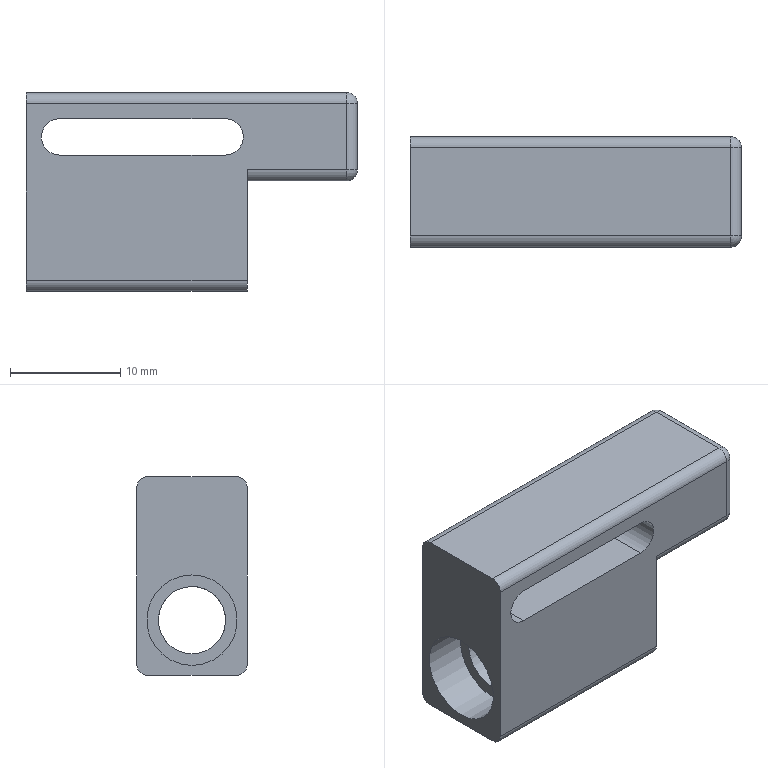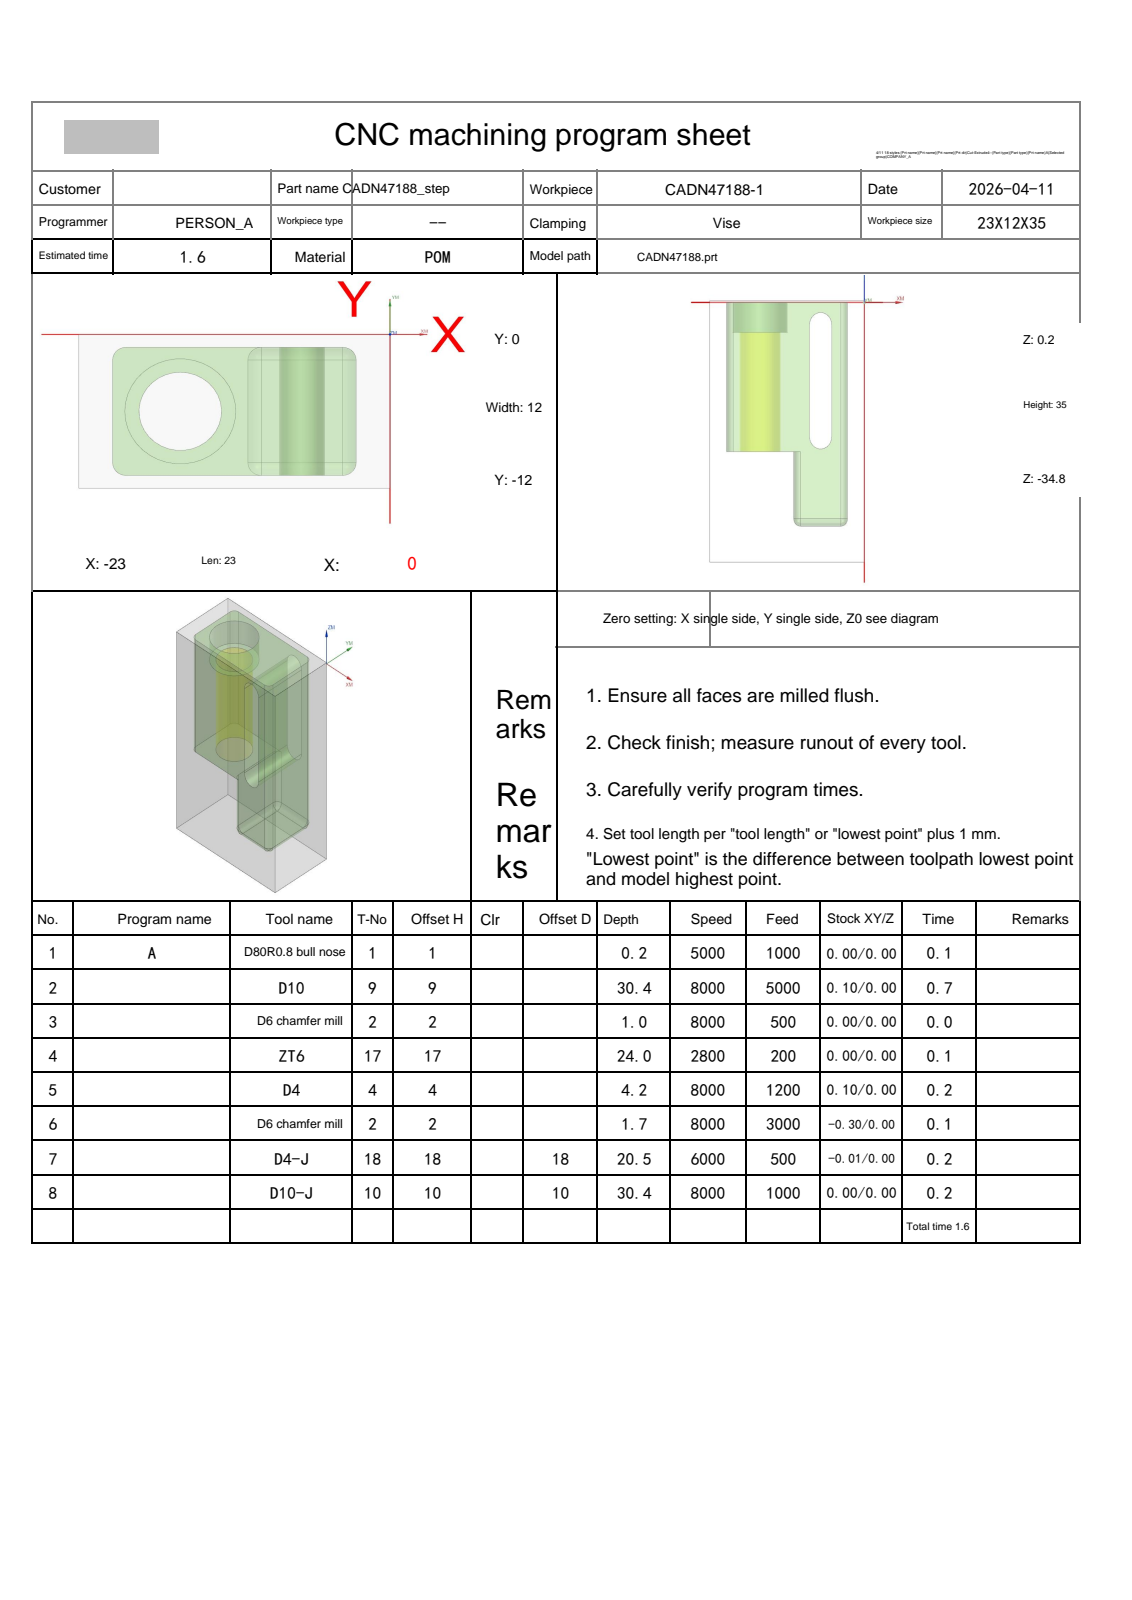NC program | NX | posted by the shop | part box 30 x 10 x 18 mm
Whole program:
%
O0001
(Machine time: 3.23 MIN)
(===Total Tool:7===)
(T1=D80R0.8 bull nose D=80.  R=0.8  D-  H01 Z=-0.   )
(T9=D10     D=10.  R=0.   D-  H09 Z=-30.2 )
(T2=D6 chamfer mill   D=6.   R=0.   D-  H02 Z=-1.5  )
(T17=ZT6    D=6.   DR_a=118 D-  H17 Z=-23.8 )
(T4=D4      D=4.   R=0.   D-  H04 Z=-4.   )
(T18=D4-J   D=4.   R=0.   D18 H18 Z=-20.3 )
(T10=D10-J  D=10.  R=0.   D10 H10 Z=-30.2 )
G80 G90 G17 G49 G40
G91 G28 Z0
M01
N1 T01 M06
(D80R0.8 bull nose  D=80. R=0.8 H=01 ce=0.00 di=0.00)
G00 G90 G54 X-65.5 Y-6. M03 S5000
G43 H01 Z20.
M08
Z2.
G01 Z0.0 F1000.
X-60.5
X37.5
X42.5
Z2.
G00 Z20.
G91 G28 Z0.0
M05
M09
G91 G28 Z0.0
M01
N2 T09 M06
(D10  D=10. R=0. H=09 ce=0.10 di=0.00)
G00 G90 G54 X-11.5 Y4.1 M03 S8000
G43 H09 Z20.
M08
Z.5
G01 X-3.5 Z.427 F5000.
G02 X2.6 Y-2. Z.34 I0.0 J-6.1
G01 Y-10. Z.267
G02 X-3.5 Y-16.1 Z.179 I-6.1 J0.0
G01 X-19.5 Z.033
G02 X-25.6 Y-10. Z-.054 I0.0 J6.1
G01 Y-2. Z-.127
G02 X-19.5 Y4.1 Z-.214 I6.1 J0.0
G01 X-3.5 Z-.36
G02 X2.6 Y-2. Z-.448 I0.0 J-6.1
G01 Y-10. Z-.52
G02 X-3.5 Y-16.1 Z-.608 I-6.1 J0.0
G01 X-19.5 Z-.754
G02 X-25.6 Y-10. Z-.841 I0.0 J6.1
G01 Y-2. Z-.914
G02 X-19.5 Y4.1 Z-1.001 I6.1 J0.0
G01 X-3.5 Z-1.147
G02 X2.6 Y-2. Z-1.235 I0.0 J-6.1
G01 Y-10. Z-1.308
G02 X-3.5 Y-16.1 Z-1.395 I-6.1 J0.0
G01 X-19.5 Z-1.541
G02 X-25.6 Y-10. Z-1.628 I0.0 J6.1
G01 Y-2. Z-1.701
G02 X-19.5 Y4.1 Z-1.789 I6.1 J0.0
G01 X-3.5 Z-1.934
G02 X2.6 Y-2. Z-2.022 I0.0 J-6.1
G01 Y-10. Z-2.095
G02 X-3.5 Y-16.1 Z-2.182 I-6.1 J0.0
G01 X-19.5 Z-2.328
G02 X-25.6 Y-10. Z-2.415 I0.0 J6.1
G01 Y-2. Z-2.488
G02 X-19.5 Y4.1 Z-2.576 I6.1 J0.0
G01 X-3.5 Z-2.722
G02 X2.6 Y-2. Z-2.809 I0.0 J-6.1
G01 Y-10. Z-2.882
G02 X-3.5 Y-16.1 Z-2.969 I-6.1 J0.0
G01 X-19.5 Z-3.115
G02 X-25.6 Y-10. Z-3.203 I0.0 J6.1
G01 Y-2. Z-3.276
G02 X-19.5 Y4.1 Z-3.363 I6.1 J0.0
G01 X-3.5 Z-3.509
G02 X2.6 Y-2. Z-3.596 I0.0 J-6.1
G01 Y-10. Z-3.669
G02 X-3.5 Y-16.1 Z-3.757 I-6.1 J0.0
G01 X-19.5 Z-3.902
G02 X-25.6 Y-10. Z-3.99 I0.0 J6.1
G01 Y-2. Z-4.063
G02 X-19.5 Y4.1 Z-4.15 I6.1 J0.0
G01 X-3.5 Z-4.296
G02 X2.6 Y-2. Z-4.383 I0.0 J-6.1
G01 Y-10. Z-4.456
G02 X-3.5 Y-16.1 Z-4.544 I-6.1 J0.0
G01 X-19.5 Z-4.69
G02 X-25.6 Y-10. Z-4.777 I0.0 J6.1
G01 Y-2. Z-4.85
G02 X-19.5 Y4.1 Z-4.937 I6.1 J0.0
G01 X-3.5 Z-5.083
G02 X2.6 Y-2. Z-5.171 I0.0 J-6.1
G01 Y-10. Z-5.244
G02 X-3.5 Y-16.1 Z-5.331 I-6.1 J0.0
G01 X-19.5 Z-5.477
G02 X-25.6 Y-10. Z-5.564 I0.0 J6.1
G01 Y-2. Z-5.637
G02 X-19.5 Y4.1 Z-5.724 I6.1 J0.0
G01 X-3.5 Z-5.87
G02 X2.6 Y-2. Z-5.958 I0.0 J-6.1
G01 Y-10. Z-6.031
G02 X-3.5 Y-16.1 Z-6.118 I-6.1 J0.0
G01 X-19.5 Z-6.264
G02 X-25.6 Y-10. Z-6.351 I0.0 J6.1
G01 Y-2. Z-6.424
G02 X-19.5 Y4.1 Z-6.512 I6.1 J0.0
G01 X-3.5 Z-6.658
G02 X2.6 Y-2. Z-6.745 I0.0 J-6.1
G01 Y-10. Z-6.818
G02 X-3.5 Y-16.1 Z-6.905 I-6.1 J0.0
G01 X-19.5 Z-7.051
G02 X-25.6 Y-10. Z-7.139 I0.0 J6.1
G01 Y-2. Z-7.211
G02 X-19.5 Y4.1 Z-7.299 I6.1 J0.0
G01 X-3.5 Z-7.445
G02 X2.6 Y-2. Z-7.532 I0.0 J-6.1
G01 Y-10. Z-7.605
G02 X-3.5 Y-16.1 Z-7.692 I-6.1 J0.0
G01 X-19.5 Z-7.838
G02 X-25.6 Y-10. Z-7.926 I0.0 J6.1
G01 Y-2. Z-7.999
G02 X-19.5 Y4.1 Z-8.086 I6.1 J0.0
G01 X-3.5 Z-8.232
G02 X2.6 Y-2. Z-8.319 I0.0 J-6.1
G01 Y-10. Z-8.392
G02 X-3.5 Y-16.1 Z-8.48 I-6.1 J0.0
G01 X-19.5 Z-8.626
G02 X-25.6 Y-10. Z-8.713 I0.0 J6.1
G01 Y-2. Z-8.786
G02 X-19.5 Y4.1 Z-8.873 I6.1 J0.0
G01 X-3.5 Z-9.019
G02 X2.6 Y-2. Z-9.106 I0.0 J-6.1
G01 Y-10. Z-9.179
G02 X-3.5 Y-16.1 Z-9.267 I-6.1 J0.0
G01 X-19.5 Z-9.413
G02 X-25.6 Y-10. Z-9.5 I0.0 J6.1
G01 Y-2. Z-9.573
G02 X-19.5 Y4.1 Z-9.66 I6.1 J0.0
G01 X-3.5 Z-9.806
G02 X2.6 Y-2. Z-9.894 I0.0 J-6.1
G01 Y-10. Z-9.967
G02 X-3.5 Y-16.1 Z-10.054 I-6.1 J0.0
G01 X-19.5 Z-10.2
G02 X-25.6 Y-10. Z-10.287 I0.0 J6.1
G01 Y-2. Z-10.36
G02 X-19.5 Y4.1 Z-10.448 I6.1 J0.0
G01 X-3.5 Z-10.593
G02 X2.6 Y-2. Z-10.681 I0.0 J-6.1
G01 Y-10. Z-10.754
G02 X-3.5 Y-16.1 Z-10.841 I-6.1 J0.0
G01 X-19.5 Z-10.987
G02 X-25.6 Y-10. Z-11.074 I0.0 J6.1
G01 Y-2. Z-11.147
G02 X-19.5 Y4.1 Z-11.235 I6.1 J0.0
G01 X-3.5 Z-11.381
G02 X2.6 Y-2. Z-11.468 I0.0 J-6.1
G01 Y-10. Z-11.541
G02 X-3.5 Y-16.1 Z-11.628 I-6.1 J0.0
G01 X-19.5 Z-11.774
G02 X-25.6 Y-10. Z-11.862 I0.0 J6.1
G01 Y-2. Z-11.935
G02 X-19.5 Y4.1 Z-12.022 I6.1 J0.0
G01 X-3.5 Z-12.168
G02 X2.6 Y-2. Z-12.255 I0.0 J-6.1
G01 Y-10. Z-12.328
G02 X-3.5 Y-16.1 Z-12.416 I-6.1 J0.0
G01 X-19.5 Z-12.561
G02 X-25.6 Y-10. Z-12.649 I0.0 J6.1
G01 Y-2. Z-12.722
G02 X-19.5 Y4.1 Z-12.809 I6.1 J0.0
G01 X-3.5 Z-12.955
G02 X2.6 Y-2. Z-13.042 I0.0 J-6.1
G01 Y-10. Z-13.115
G02 X-3.5 Y-16.1 Z-13.203 I-6.1 J0.0
G01 X-19.5 Z-13.349
G02 X-25.6 Y-10. Z-13.436 I0.0 J6.1
G01 Y-2. Z-13.509
G02 X-19.5 Y4.1 Z-13.596 I6.1 J0.0
G01 X-3.5 Z-13.742
G02 X2.6 Y-2. Z-13.83 I0.0 J-6.1
G01 Y-10. Z-13.903
G02 X-3.5 Y-16.1 Z-13.99 I-6.1 J0.0
G01 X-19.5 Z-14.136
G02 X-25.6 Y-10. Z-14.223 I0.0 J6.1
G01 Y-2. Z-14.296
G02 X-19.5 Y4.1 Z-14.383 I6.1 J0.0
G01 X-3.5 Z-14.529
G02 X2.6 Y-2. Z-14.617 I0.0 J-6.1
G01 Y-10. Z-14.69
G02 X-3.5 Y-16.1 Z-14.777 I-6.1 J0.0
G01 X-19.5 Z-14.923
G02 X-25.6 Y-10. Z-15.01 I0.0 J6.1
G01 Y-2. Z-15.083
G02 X-19.5 Y4.1 Z-15.171 I6.1 J0.0
G01 X-3.5 Z-15.317
G02 X2.6 Y-2. Z-15.404 I0.0 J-6.1
G01 Y-10. Z-15.477
G02 X-3.5 Y-16.1 Z-15.564 I-6.1 J0.0
G01 X-19.5 Z-15.71
G02 X-25.6 Y-10. Z-15.798 I0.0 J6.1
G01 Y-2. Z-15.87
G02 X-19.5 Y4.1 Z-15.958 I6.1 J0.0
G01 X-3.5 Z-16.104
G02 X2.6 Y-2. Z-16.191 I0.0 J-6.1
G01 Y-10. Z-16.264
G02 X-3.5 Y-16.1 Z-16.351 I-6.1 J0.0
G01 X-19.5 Z-16.497
G02 X-25.6 Y-10. Z-16.585 I0.0 J6.1
G01 Y-2. Z-16.658
G02 X-19.5 Y4.1 Z-16.745 I6.1 J0.0
G01 X-3.5 Z-16.891
G02 X2.6 Y-2. Z-16.978 I0.0 J-6.1
G01 Y-10. Z-17.051
G02 X-3.5 Y-16.1 Z-17.139 I-6.1 J0.0
G01 X-19.5 Z-17.284
G02 X-25.6 Y-10. Z-17.372 I0.0 J6.1
G01 Y-2. Z-17.445
G02 X-19.5 Y4.1 Z-17.532 I6.1 J0.0
G01 X-3.5 Z-17.678
G02 X2.6 Y-2. Z-17.765 I0.0 J-6.1
G01 Y-10. Z-17.838
G02 X-3.5 Y-16.1 Z-17.926 I-6.1 J0.0
G01 X-19.5 Z-18.072
G02 X-25.6 Y-10. Z-18.159 I0.0 J6.1
G01 Y-2. Z-18.232
G02 X-19.5 Y4.1 Z-18.319 I6.1 J0.0
G01 X-3.5 Z-18.465
G02 X2.6 Y-2. Z-18.553 I0.0 J-6.1
G01 Y-10. Z-18.626
G02 X-3.5 Y-16.1 Z-18.713 I-6.1 J0.0
G01 X-19.5 Z-18.859
G02 X-25.6 Y-10. Z-18.946 I0.0 J6.1
G01 Y-2. Z-19.019
G02 X-19.5 Y4.1 Z-19.107 I6.1 J0.0
G01 X-3.5 Z-19.252
G02 X2.6 Y-2. Z-19.34 I0.0 J-6.1
G01 Y-10. Z-19.413
G02 X-3.5 Y-16.1 Z-19.5 I-6.1 J0.0
G01 X-19.5 Z-19.646
G02 X-25.6 Y-10. Z-19.733 I0.0 J6.1
G01 Y-2. Z-19.806
G02 X-19.5 Y4.1 Z-19.894 I6.1 J0.0
G01 X-3.5 Z-20.04
G02 X2.6 Y-2. Z-20.127 I0.0 J-6.1
G01 Y-10. Z-20.2
G02 X-3.5 Y-16.1 Z-20.287 I-6.1 J0.0
G01 X-19.5 Z-20.433
G02 X-25.6 Y-10. Z-20.521 I0.0 J6.1
G01 Y-2. Z-20.594
G02 X-19.5 Y4.1 Z-20.681 I6.1 J0.0
G01 X-3.5 Z-20.827
G02 X2.6 Y-2. Z-20.914 I0.0 J-6.1
G01 Y-10. Z-20.987
G02 X-3.5 Y-16.1 Z-21.074 I-6.1 J0.0
G01 X-19.5 Z-21.22
G02 X-25.6 Y-10. Z-21.308 I0.0 J6.1
G01 Y-2. Z-21.381
G02 X-19.5 Y4.1 Z-21.468 I6.1 J0.0
G01 X-3.5 Z-21.614
G02 X2.6 Y-2. Z-21.701 I0.0 J-6.1
G01 Y-10. Z-21.774
G02 X-3.5 Y-16.1 Z-21.862 I-6.1 J0.0
G01 X-19.5 Z-22.008
G02 X-25.6 Y-10. Z-22.095 I0.0 J6.1
G01 Y-2. Z-22.168
G02 X-19.5 Y4.1 Z-22.255 I6.1 J0.0
G01 X-3.5 Z-22.401
G02 X2.6 Y-2. Z-22.489 I0.0 J-6.1
G01 Y-10. Z-22.561
G02 X-3.5 Y-16.1 Z-22.649 I-6.1 J0.0
G01 X-19.5 Z-22.795
G02 X-25.6 Y-10. Z-22.882 I0.0 J6.1
G01 Y-2. Z-22.955
G02 X-19.5 Y4.1 Z-23.042 I6.1 J0.0
G01 X-3.5 Z-23.188
G02 X2.6 Y-2. Z-23.276 I0.0 J-6.1
G01 Y-10. Z-23.349
G02 X-3.5 Y-16.1 Z-23.436 I-6.1 J0.0
G01 X-19.5 Z-23.582
G02 X-25.6 Y-10. Z-23.669 I0.0 J6.1
G01 Y-2. Z-23.742
G02 X-19.5 Y4.1 Z-23.83 I6.1 J0.0
G01 X-3.5 Z-23.976
G02 X2.6 Y-2. Z-24.063 I0.0 J-6.1
G01 Y-10. Z-24.136
G02 X-3.5 Y-16.1 Z-24.223 I-6.1 J0.0
G01 X-19.5 Z-24.369
G02 X-25.6 Y-10. Z-24.456 I0.0 J6.1
G01 Y-2. Z-24.529
G02 X-19.5 Y4.1 Z-24.617 I6.1 J0.0
G01 X-3.5 Z-24.763
G02 X2.6 Y-2. Z-24.85 I0.0 J-6.1
G01 Y-10. Z-24.923
G02 X-3.5 Y-16.1 Z-25.01 I-6.1 J0.0
G01 X-19.5 Z-25.156
G02 X-25.6 Y-10. Z-25.244 I0.0 J6.1
G01 Y-2. Z-25.317
G02 X-19.5 Y4.1 Z-25.404 I6.1 J0.0
G01 X-3.5 Z-25.55
G02 X2.6 Y-2. Z-25.637 I0.0 J-6.1
G01 Y-10. Z-25.71
G02 X-3.5 Y-16.1 Z-25.798 I-6.1 J0.0
G01 X-19.5 Z-25.943
G02 X-25.6 Y-10. Z-26.031 I0.0 J6.1
G01 Y-2. Z-26.104
G02 X-19.5 Y4.1 Z-26.191 I6.1 J0.0
G01 X-3.5 Z-26.337
G02 X2.6 Y-2. Z-26.424 I0.0 J-6.1
G01 Y-10. Z-26.497
G02 X-3.5 Y-16.1 Z-26.585 I-6.1 J0.0
G01 X-19.5 Z-26.731
G02 X-25.6 Y-10. Z-26.818 I0.0 J6.1
G01 Y-2. Z-26.891
G02 X-19.5 Y4.1 Z-26.978 I6.1 J0.0
G01 X-3.5 Z-27.124
G02 X2.6 Y-2. Z-27.212 I0.0 J-6.1
G01 Y-10. Z-27.285
G02 X-3.5 Y-16.1 Z-27.372 I-6.1 J0.0
G01 X-19.5 Z-27.518
G02 X-25.6 Y-10. Z-27.605 I0.0 J6.1
G01 Y-2. Z-27.678
G02 X-19.5 Y4.1 Z-27.766 I6.1 J0.0
G01 X-3.5 Z-27.911
G02 X2.6 Y-2. Z-27.999 I0.0 J-6.1
G01 Y-10. Z-28.072
G02 X-3.5 Y-16.1 Z-28.159 I-6.1 J0.0
G01 X-19.5 Z-28.305
G02 X-25.6 Y-10. Z-28.392 I0.0 J6.1
G01 Y-2. Z-28.465
G02 X-19.5 Y4.1 Z-28.553 I6.1 J0.0
G01 X-3.5 Z-28.699
G02 X2.6 Y-2. Z-28.786 I0.0 J-6.1
G01 Y-10. Z-28.859
G02 X-3.5 Y-16.1 Z-28.946 I-6.1 J0.0
G01 X-19.5 Z-29.092
G02 X-25.6 Y-10. Z-29.18 I0.0 J6.1
G01 Y-2. Z-29.253
G02 X-19.5 Y4.1 Z-29.34 I6.1 J0.0
G01 X-3.5 Z-29.486
G02 X2.6 Y-2. Z-29.573 I0.0 J-6.1
G01 Y-10. Z-29.646
G02 X-3.5 Y-16.1 Z-29.733 I-6.1 J0.0
G01 X-19.5 Z-29.879
G02 X-25.6 Y-10. Z-29.967 I0.0 J6.1
G01 Y-2. Z-30.04
G02 X-19.5 Y4.1 Z-30.127 I6.1 J0.0
G01 X-11.5 Z-30.2
X-3.5
G02 X2.6 Y-2. I0.0 J-6.1
G01 Y-10.
G02 X-3.5 Y-16.1 I-6.1 J0.0
G01 X-19.5
G02 X-25.6 Y-10. I0.0 J6.1
G01 Y-2.
G02 X-19.5 Y4.1 I6.1 J0.0
G01 X-11.5
X-11.
Z-29.2
G00 Z20.
G91 G28 Z0.0
M05
M09
G91 G28 Z0.0
M01
N3 T02 M06
(D6 chamfer mill  D=6. R=0. H=02 ce=0.00 di=0.00)
G00 G90 G54 X-15.5 Y-6. M03 S8000
G43 H02 Z20.
M08
G98 G81 X-15.5 Y-6. Z-.8 R1. F500.
G80
G00 Z20.
G91 G28 Z0.0
M05
M09
G91 G28 Z0.0
M01
N4 T17 M06
(ZT6 D=6. DR_a=118 H=17)
G00 G90 G54 X-15.5 Y-6. M03 S2800
G43 H17 Z20.
M08
G98 G83 X-15.5 Y-6. Z-23.803 R1. F200. Q2.
G80
G00 Z20.
G91 G28 Z0.0
M05
M09
G91 G28 Z0.0
M01
N5 T04 M06
(D4  D=4. R=0. H=04 ce=0.10 di=0.00)
G00 G90 G54 X-15.5 Y-6. M03 S8000
G43 H04 Z20.
M08
Z.5
G03 X-14.5 Y-5. I0.0 J1. F1200.
X-15.5 Y-4. I-1. J0.0
X-15.5 Y-4. Z.2 I0.0 J-2.
X-15.5 Y-4. Z-.1 I0.0 J-2.
X-15.5 Y-4. Z-.4 I0.0 J-2.
X-15.5 Y-4. Z-.7 I0.0 J-2.
X-15.5 Y-4. Z-1. I0.0 J-2.
X-15.5 Y-4. Z-1.3 I0.0 J-2.
X-15.5 Y-4. Z-1.6 I0.0 J-2.
X-15.5 Y-4. Z-1.9 I0.0 J-2.
X-15.5 Y-4. Z-2.2 I0.0 J-2.
X-15.5 Y-4. Z-2.5 I0.0 J-2.
X-15.5 Y-4. Z-2.8 I0.0 J-2.
X-15.5 Y-4. Z-3.1 I0.0 J-2.
X-15.5 Y-4. Z-3.4 I0.0 J-2.
X-15.5 Y-4. Z-3.7 I0.0 J-2.
X-15.5 Y-4. Z-4. I0.0 J-2.
X-17.5 Y-6. I0.0 J-2.
X-15.5 Y-8. I2. J0.0
X-13.5 Y-6. I0.0 J2.
X-15.5 Y-4. I-2. J0.0
X-16.5 Y-5. I0.0 J-1.
X-15.5 Y-6. I1. J0.0
G00 Z20.
G91 G28 Z0.0
M05
M09
G91 G28 Z0.0
M01
N6 T02 M06
(D6 chamfer mill  D=6. R=0. H=02 ce=0.00 di=0.00)
G00 G90 G54 X-11.25 Y-13.128 M03 S8000
G43 H02 Z20.
M08
Z2.099
G01 Z-1.5 F3000.
G03 X-11.17 Y-12.828 I-.52 J.3
X-11.47 Y-12.308 I-.6 J0.0
G01 X-11.5 Y-12.3
X-19.5
G02 X-21.8 Y-10. I0.0 J2.3
G01 Y-2.
G02 X-19.5 Y.3 I2.3 J0.0
G01 X-3.5
G02 X-1.2 Y-2. I0.0 J-2.3
G01 Y-10.
G02 X-3.5 Y-12.3 I-2.3 J0.0
G01 X-11.5
X-11.53 Y-12.308
G03 X-11.83 Y-12.828 I.3 J-.52
X-11.75 Y-13.128 I.6 J0.0
G01 Z2.099
G00 Z20.
G00 G90 X-12.267 Y-4.949 M03 S8000
Z20.
Z2.5
G01 X-12.384 Y-4.631 Z2.377 F500.
X-12.568 Y-4.273 Z2.23
X-12.792 Y-3.939 Z2.084
X-13.054 Y-3.634 Z1.937
X-13.35 Y-3.362 Z1.791
X-13.676 Y-3.127 Z1.645
X-13.924 Y-2.984 Z1.541
X-14.291 Y-2.819 Z1.394
X-14.674 Y-2.699 Z1.248
X-15.07 Y-2.624 Z1.101
X-15.471 Y-2.597 Z.955
X-15.873 Y-2.617 Z.809
X-16.269 Y-2.685 Z.662
X-16.655 Y-2.799 Z.516
X-17.024 Y-2.958 Z.37
X-17.373 Y-3.159 Z.223
X-17.695 Y-3.399 Z.077
X-17.986 Y-3.677 Z-.07
X-18.243 Y-3.986 Z-.216
X-18.462 Y-4.324 Z-.362
X-18.639 Y-4.685 Z-.509
X-18.772 Y-5.064 Z-.655
X-18.859 Y-5.457 Z-.802
X-18.9 Y-5.857 Z-.948
Y-6. Z-1.
G03 X-15.5 Y-9.4 I3.4 J0.0
X-12.1 Y-6. I0.0 J3.4
X-15.5 Y-2.6 I-3.4 J0.0
X-18.9 Y-6. I0.0 J-3.4
X-18.863 Y-6.498 I3.4 J0.0
G01 Z1.5
G00 Z20.
G91 G28 Z0.0
M05
M09
G91 G28 Z0.0
M01
N7 T18 M06
(D4-J  D=4. R=0. H=18 ce=-0.01 di=0.00)
G00 G90 G54 X-16.344 Y-5.2 M03 S6000
G43 H18 Z10.2
M08
Z-3.
G01 Z-4. F500.
G41 D18
X-16.815
G03 X-17.615 Y-6. I0.0 J-.8
X-15.5 Y-8.115 I2.115 J0.0
X-13.385 Y-6. I0.0 J2.115
X-15.5 Y-3.885 I-2.115 J0.0
X-17.615 Y-6. I0.0 J-2.115
X-17.577 Y-6.398 I2.115 J0.0
X-16.792 Y-7.047 I.786 J.15
G01 X-16.641 Y-7.033
X-16.375 Y-6.982
G40 X-16.178 Y-6.944
Z-3.
G00 Z10.2
G00 G90 X-15.785 Y-5.632 M03 S6000
Z10.2
Z-6.575
G01 Z-8.075 F300.
G41 D18
X-15.965 Y-5.4
G03 X-16.565 Y-6. I0.0 J-.6
X-15.5 Y-7.065 I1.065 J0.0
X-14.435 Y-6. I0.0 J1.065
X-15.5 Y-4.935 I-1.065 J0.0
X-16.565 Y-6. I0.0 J-1.065
X-16.491 Y-6.391 I1.065 J0.0
X-15.933 Y-6.771 I.558 J.22
X-15.712 Y-6.729 I0.0 J.6
G01 G40 X-15.63 Y-6.446
Z-6.575
G00 X-15.785 Y-5.632
Z-10.65
G01 Z-12.15
G41 D18
X-15.965 Y-5.4
G03 X-16.565 Y-6. I0.0 J-.6
X-15.5 Y-7.065 I1.065 J0.0
X-14.435 Y-6. I0.0 J1.065
X-15.5 Y-4.935 I-1.065 J0.0
X-16.565 Y-6. I0.0 J-1.065
X-16.491 Y-6.391 I1.065 J0.0
X-15.933 Y-6.771 I.558 J.22
X-15.712 Y-6.729 I0.0 J.6
G01 G40 X-15.63 Y-6.446
Z-10.65
G00 X-15.785 Y-5.632
Z-14.725
G01 Z-16.225
G41 D18
X-15.965 Y-5.4
G03 X-16.565 Y-6. I0.0 J-.6
X-15.5 Y-7.065 I1.065 J0.0
X-14.435 Y-6. I0.0 J1.065
X-15.5 Y-4.935 I-1.065 J0.0
X-16.565 Y-6. I0.0 J-1.065
X-16.491 Y-6.391 I1.065 J0.0
X-15.933 Y-6.771 I.558 J.22
X-15.712 Y-6.729 I0.0 J.6
G01 G40 X-15.63 Y-6.446
Z-14.725
G00 X-15.785 Y-5.632
Z-18.8
G01 Z-20.3
G41 D18
X-15.965 Y-5.4
G03 X-16.565 Y-6. I0.0 J-.6
X-15.5 Y-7.065 I1.065 J0.0
X-14.435 Y-6. I0.0 J1.065
X-15.5 Y-4.935 I-1.065 J0.0
X-16.565 Y-6. I0.0 J-1.065
X-16.491 Y-6.391 I1.065 J0.0
X-15.933 Y-6.771 I.558 J.22
X-15.712 Y-6.729 I0.0 J.6
G01 G40 X-15.63 Y-6.446
Z-18.8
G00 Z10.2
G91 G28 Z0.0
M05
M09
G91 G28 Z0.0
M01
N8 T10 M06
(D10-J  D=10. R=0. H=10 ce=0.00 di=0.00)
G00 G90 G54 X-20.512 Y5.128 M03 S8000
G43 H10 Z20.
M08
Z-14.6
G01 Z-15.1 F1000.
G41 D10
X-20.497 Y4.929
G03 X-19.5 Y4. I.997 J.071
G01 X-3.5
G02 X2.5 Y-2. I0.0 J-6.
G01 Y-10.
G02 X-3.5 Y-16. I-6. J0.0
G01 X-19.5
G02 X-25.5 Y-10. I0.0 J6.
G01 Y-2.
G02 X-19.5 Y4. I6. J0.0
G01 X-19.
G03 X-18. Y5. I0.0 J1.
G01 G40 Y5.2
Z-14.6
G00 Z20.
X-20.512 Y5.128
Z-29.7
G01 Z-30.2
G41 D10
X-20.497 Y4.929
G03 X-19.5 Y4. I.997 J.071
G01 X-3.5
G02 X2.5 Y-2. I0.0 J-6.
G01 Y-10.
G02 X-3.5 Y-16. I-6. J0.0
G01 X-19.5
G02 X-25.5 Y-10. I0.0 J6.
G01 Y-2.
G02 X-19.5 Y4. I6. J0.0
G01 X-19.
G03 X-18. Y5. I0.0 J1.
G01 G40 Y5.2
Z-29.7
G00 Z20.
M05
M09
G91 G28 Z0.0
G91 G28 Y0.0
M30
%